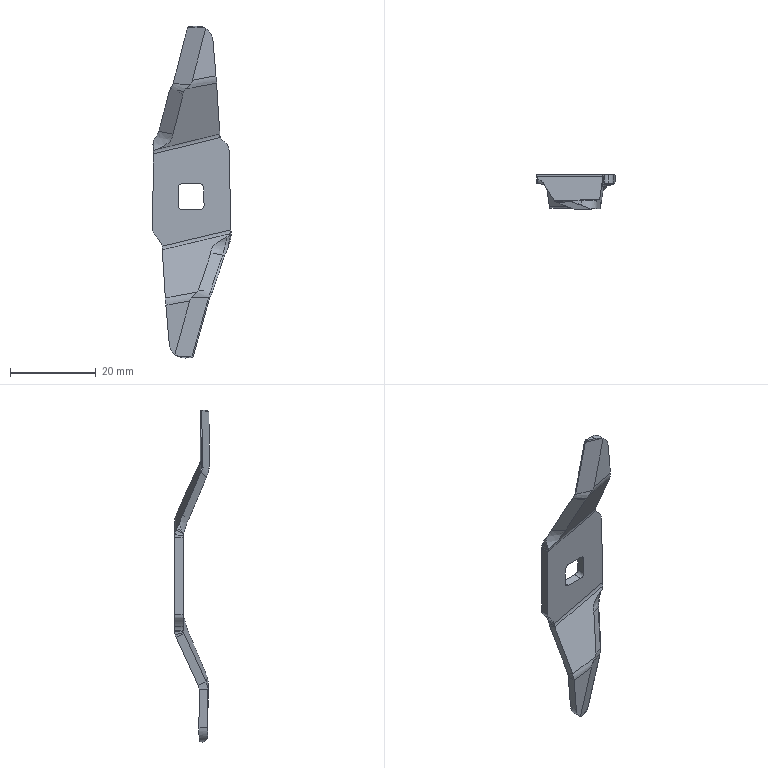Part | SolidWorks | features 3DProfileFeature 4, SM3dBend 4, SweepCut 2, Cut 1, Fillet 1, FlatPattern 1, SMBaseFlange 1, SheetMetal 1 | 1 solid | 83 faces | box 18.18 x 8.128 x 77.268 mm | volume 1719 mm3 | plane 40 | cylinder 24 | spline 19 | commonest cylinder face diameters 4 x4 8 x4 2 x3 2.001 x2 1 x1 1.05 x1